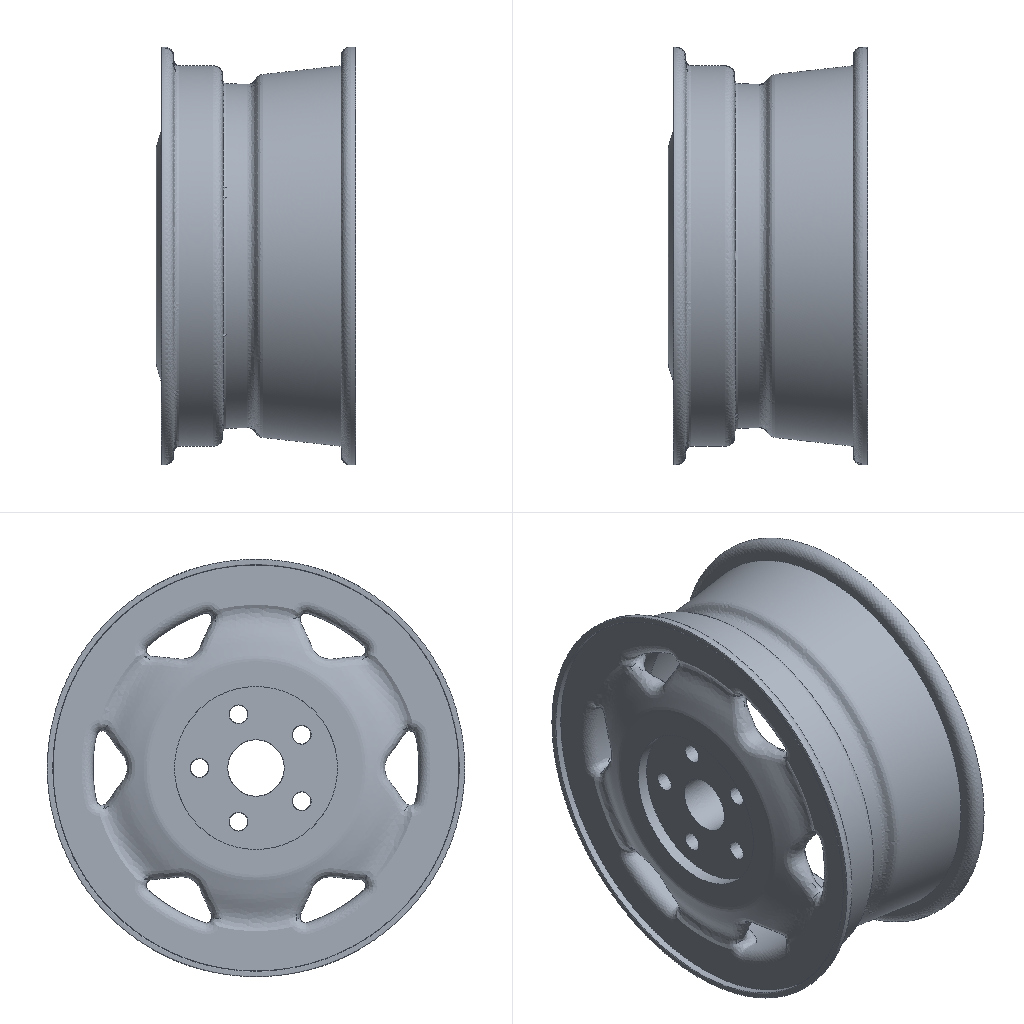Simulation study
Set-up summary:
category,name,step,type,value,unit,region
solver,ansys_mapdl
solver,version,,,22.2
units,MPA,,stated
analysis,deck,,static,static
load_step,requested,,,1
analysis,nlgeom,,,False
mesh,nodes,,,699764
mesh,elements,,,407594
element_type,ANSYS 187 (type 1),,solid,405382
element_type,ANSYS 174 (type 2),,contact,2212
element_type,ANSYS 170 (type 3),,target,0
load,load commands in deck,,count,3
bc,support commands in deck,,count,1
named_set,_FIXEDSU,,component
material,1,,in results
check,setup vs results,,match,results also hold 0 node(s) and 1 element(s) the deck makes with ['EN']; those were not compared; 1 setup node(s) no element uses are not in the results (e.g. [699763]); 1 node(s) the solver created internally for pilot nodes (solve.out) are in the results only
Ansys APDL input file, long lists of numbers shortened:
/batch
/config,noeldb,1     ! force off writing results to database
*get,_wallstrt,active,,time,wall
! ANSYS input file written by Workbench version 2022 R2
! File used for geometry attach: D:\虚拟C盘\建+仿+论\38.轮毂\零件33.STEP
/title,_____--____ (A5)
! ****** Begin Custom Load Command Snippet ******
/COM, ACT Extensions:
/COM,     LSDYNA, 2022.2
/COM,/COM,     ANSYSMotion, 2022.2
/COM,
! ****** End   Custom Load Command Snippet ******
*DIM,_wb_ProjectScratch_dir,string,248
_wb_ProjectScratch_dir(1) = 'D:\虚拟C盘\建+仿+论\_ProjectScratch\Scr2DDF\'
*DIM,_wb_SolverFiles_dir,string,248
_wb_SolverFiles_dir(1) = 'D:\虚拟C盘\建+仿+论\径向力分析_files\dp0\SYS\MECH\'
*DIM,_wb_userfiles_dir,string,248
_wb_userfiles_dir(1) = 'D:\虚拟C盘\建+仿+论\径向力分析_files\user_files\'
/com,--- Data in consistent NMM units. See Solving Units in the help system for more information.
/units,MPA
/nopr
/wb,file,start              !  signify a WB generated input file
/prep7
! Turn off shape checking because checks already performed inside WB mesher.
! See help system for more information.
SHPP,OFF,,NOWARN
/nolist
etcon,set             ! allow ANSYS to choose best KEYOP's for 180x elements, resets any applicable keyopt to MAPDL defaults
/com,*********** Nodes for the whole assembly ***********
nblock,3,,769738
(1i9,3e20.9e3)
        1    -1.194508278E+02     0.000000000E+00     1.822860838E+02
! (699761 more lines like these left out)
-1
/com,*********** Nodes for all Remote Points ***********
nblock,3
(1i9,3e20.9e3)
   699763    -1.736000000E+03     0.000000000E+00     0.000000000E+00
   699764    -1.761534958E+02     0.000000000E+00    -1.805667084E-16
-1
/wb,elem,start            !  set before creation of elements
/com,*********** Elements for Body 1 "__33-FreeParts|__3" ***********
et,1,187
eblock,19,solid,,405382
(19i9)
        1        1        1        1        0        0        0        0       10        0        1    18217    26073   107494    96537   239457   282725   239461   239459
! (810763 more lines like these left out)
-1
/wb,elem,end               !  done creating elements
/com,*********** Send User Defined Coordinate System(s) ***********
csys,0
toffst,273.15,  ! Temperature offset from absolute zero
/com,*********** Set Reference Temperature ***********
tref,22.
/wb,mat,start              !  starting to send materials
/com,*********** Send Materials ***********
Temperature = 'TEMP' ! Temperature
MP,DENS,1,2.77e-09,	! tonne mm^-3
MP,ALPX,1,2.3e-05,	! C^-1
MP,C,1,875000000,	! mm^2 s^-2 C^-1
MPTEMP,,,,,,,,
MPTEMP,1,-100
MPTEMP,2,0
MPTEMP,3,100
MPTEMP,4,200
MPDATA,KXX,1, ,114,144,165,175,	! tonne mm s^-3 C^-1
MPTEMP,,,,,,,,
MPTEMP,,,,,,,,
MPTEMP,1,0
MPTEMP,2,20
MPTEMP,3,100
MPDATA,RSVX,1, ,2.43e-05,2.67e-05,3.63e-05,	! ohm mm
MPTEMP,,,,,,,,
MP,EX,1,71000,	! tonne s^-2 mm^-1
MP,NUXY,1,0.33,
MP,MURX,1,1,
/wb,mat,end                !  done sending materials
!************************* Model Summary ********************
!__33-FreeParts|__3,	铝合金,	matid,	1
!************************* End Model Summary ********************
! get the diagonal of the bounding box. Needed later for other things
*get,_xmin,node,,mnloc,x
*get,_ymin,node,,mnloc,y
*get,_zmin,node,,mnloc,z
*get,_xmax,node,,mxloc,x
*get,_ymax,node,,mxloc,y
*get,_zmax,node,,mxloc,z
_ASMDIAG=(_xmax-_xmin)*(_xmax-_xmin)+(_ymax-_ymin)*(_ymax-_ymin)+(_zmax-_zmin)*(_zmax-_zmin)
_ASMDIAG=SQRT(_ASMDIAG)
/wb,contact,start          !  starting to send contact
/wb,contact,end            !  done creating contacts
/golist
/wb,load,start             !  starting to send loads
/com,*********** Fixed Supports ***********
CMBLOCK,_FIXEDSU,NODE,    88573
(8i10)
      4243      4245      4246      4247      4248      4249      4250      4251
! (11071 more lines like these left out)
cmsel,s,_FIXEDSU
d,all,all
nsel,all
/com,*********** Create Remote Point "内部远程点 2" ***********
! -------- Remote Point Used by "力矩" --------
*set,tid,3
*set,cid,2
et,cid,174
et,tid,170
keyo,tid,2,1               ! Don't fix the pilot node
keyo,tid,4,111111
keyo,cid,12,5              ! Bonded Contact
keyo,cid,4,1               ! Deformable RBE3 style load
keyo,cid,2,2               ! MPC style contact
eblock,10,,,2212
(15i9)
   560503        2        2        2        0    11022    11023    74110    74110   190159   190166    74110   190160
! (2211 more lines like these left out)
-1
*set,_npilot,699764
_npilot62=_npilot
type,tid
mat ,cid
real,cid
tshape,pilo
en,562715,_npilot
tshape
/com,*********** Construct Moment Using Remote Attachment ***********
/gst,on,on
fini
*get,_numnode,node,0,count
*get,_numelem,elem,0,count
*get, _MAXELEMNUM, elem, 0, NUM, MAX
*get, _MAXNODENUM, node, 0, NUM, MAX
*get, _MAXELEMTYPE, etyp, 0, NUM, MAX
*get, _MAXREALCONST, rcon, 0, NUM, MAX
/go
/wb,load,end               !  done creating loads
/com,--- Number of total nodes = %_numnode%
/com,--- Number of contact elements = 2212
/com,--- Number of spring elements = 0
/com,--- Number of bearing elements = 0
/com,--- Number of solid elements = 405382
/com,--- Number of condensed parts = 0
/com,--- Number of total elements = %_numelem%
*get,_wallbsol,active,,time,wall
/com,****************************************************************************
/com,*************************    SOLUTION       ********************************
/com,****************************************************************************
/solu
antype,0                   ! static analysis
_thickRatio=  1     ! Ratio of thick parts in the model
eqsl,pcg,1e-8,,,,,,1
cntr,print,1               ! print out contact info and also make no initial contact an error
dmpoption,emat,no             ! Don't combine emat file for DANSYS
dmpoption,esav,no             ! Don't combine esav file for DANSYS
nldiag,cont,iter           ! print out contact info each equilibrium iteration
rescontrol,,none                 ! Do not keep any restart files
/com,****************************************************
/com,******************* SOLVE FOR LS 1 OF 1 ****************
nsel,s,node,,699764
f,all,mx,1736000.
f,all,my,0.
f,all,mz,0.
nsel,all
/nopr
/gopr
nsub,1,1,1
time,1.
outres,erase
outres,all,none
outres,nsol,all,
outres,rsol,all
outres,eangl,all
outres,etmp,all
outres,veng,all
outres,strs,all,
outres,epel,all,
outres,eppl,all,
outres,cont,all,
! *********** WB SOLVE COMMAND ***********
! check interactive state
*get,ANSINTER_,active,,int
*if,ANSINTER_,ne,0,then
/eof
*endif
solve
/com *************** Write FE CONNECTORS *********
CEWRITE,file,ce,,INTE
/com,****************************************************
/com,*************** FINISHED SOLVE FOR LS 1 *************
*get,_wallasol,active,,time,wall
/nopr
*get,_numnode,node,0,count
*get,_numelem,elem,0,count
*get, _MAXELEMNUM, elem, 0, NUM, MAX
*get, _MAXNODENUM, node, 0, NUM, MAX,,,INTERNAL
*get, _MAXELEMTYPE, etyp, 0, NUM, MAX
*get, _MAXREALCONST, rcon, 0, NUM, MAX
*get,_NSOLTHREADS,active,0,ntfs
*get,_NSOLPROCESSES,active,0,npfs
/gopr
*get,_PCGITER,active,,solu,cgiter
/post1
xmlo,ENCODING,ISO-8859-1
xmlo,parm
/xml,parm,xml
fini
/gopr
*get,_walldone,active,,time,wall
_preptime=(_wallbsol-_wallstrt)*3600
_solvtime=(_wallasol-_wallbsol)*3600
_posttime=(_walldone-_wallasol)*3600
_totaltim=(_walldone-_wallstrt)*3600
*get,_dlbratio,active,0,solu,dlbr
*get,_combtime,active,0,solu,comb
*get,_ssmode,active,0,solu,ssmm
*get,_ndofs,active,0,solu,ndof
*get,_sol_end_time,active,0,set,time
*if,_sol_end_time,eq,1.,then
/fclean				!clean distributed files
*endif
/com,--- Total number of nodes = %_numnode%
/com,--- Total number of elements = %_numelem%
/com,--- Element load balance ratio = %_dlbratio%
/com,--- Time to combine distributed files = %_combtime%
/com,--- Sparse memory mode = %_ssmode%
/com,--- Number of DOF = %_ndofs%
/wb,file,end               ! done with WB generated input
Results summary:
result,analysis,,,static
result,last_loadstep,,,1
result,primary field,,,displacement
result,reaction total,1,FX,-2e-06,N
result,reaction total,1,FY,-3e-06,N
result,reaction total,1,FZ,1e-05,N
result,mass,,,0.01761,"NMM: mm, ton, N, s, mV, mA, degC"